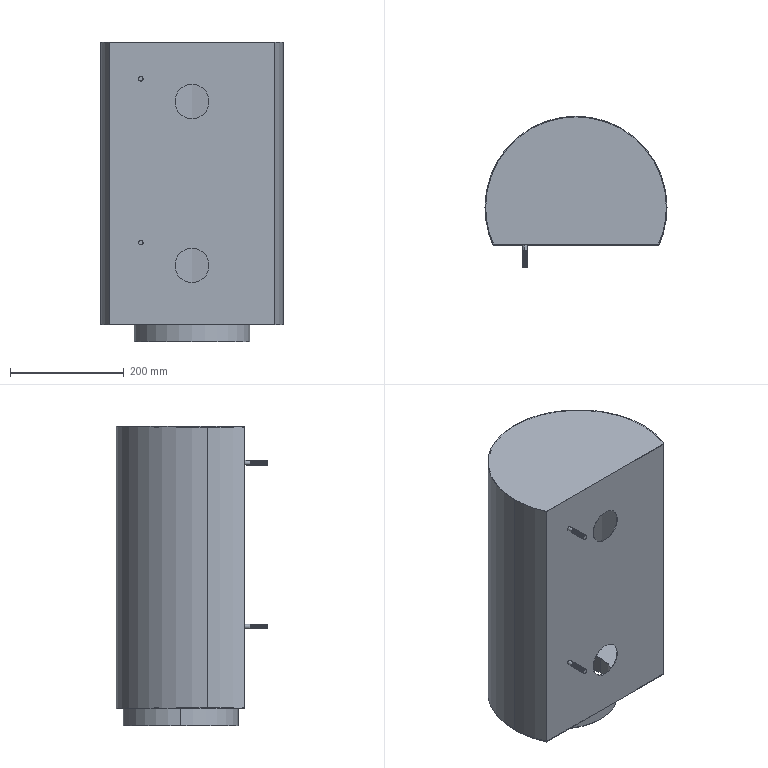Part | SolidWorks | features ICE 6, SweepThread 2, Extrusion 1, Shell 1 | 1 solid | 157 faces | box 320 x 266 x 526 mm | volume 676620 mm3 | cylinder 138 | plane 13 | spline 6 | commonest cylinder face diameters 8 x124 60 x4 317.6 x3 320 x3 200 x2 202.4 x2